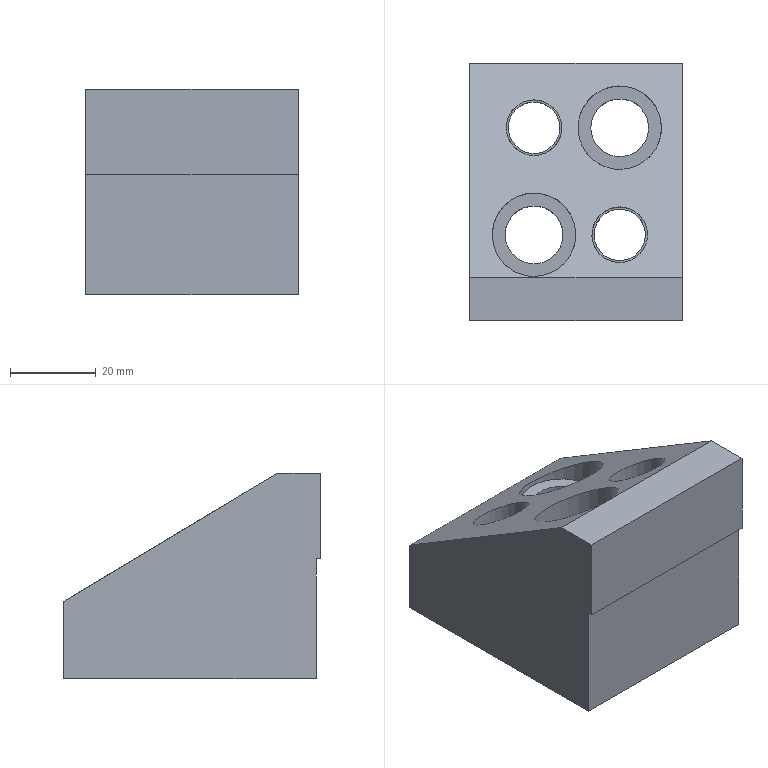Part | NX | features solid 2 | 1 solid | 21 faces | box 49.578 x 60 x 48 mm | volume 81453 mm3 | plane 13 | cylinder 8 | commonest cylinder face diameters 12 x2 13 x2 13.5 x2 19.5 x2
STEP:
#1=CARTESIAN_POINT('',(-469.,120.,-55.));
#2=VERTEX_POINT('',#1);
#3=CARTESIAN_POINT('',(-475.,120.,-55.));
#4=DIRECTION('',(0.,0.,1.));
#5=DIRECTION('',(1.,0.,0.));
#6=AXIS2_PLACEMENT_3D('',#3,#4,#5);
#7=CIRCLE('',#6,6.);
#8=EDGE_CURVE('',#2,#2,#7,.F.);
#9=ORIENTED_EDGE('',*,*,#8,.F.);
#10=EDGE_LOOP('',(#9));
#11=FACE_BOUND('',#10,.T.);
#12=CARTESIAN_POINT('',(-489.,145.,-55.));
#13=VERTEX_POINT('',#12);
#14=CARTESIAN_POINT('',(-495.,145.,-55.));
#15=DIRECTION('',(0.,0.,1.));
#16=DIRECTION('',(1.,0.,0.));
#17=AXIS2_PLACEMENT_3D('',#14,#15,#16);
#18=CIRCLE('',#17,6.);
#19=EDGE_CURVE('',#13,#13,#18,.F.);
#20=ORIENTED_EDGE('',*,*,#19,.F.);
#21=EDGE_LOOP('',(#20));
#22=FACE_BOUND('',#21,.T.);
#23=CARTESIAN_POINT('',(-468.25,145.,-55.));
#24=VERTEX_POINT('',#23);
#25=CARTESIAN_POINT('',(-475.,145.,-55.));
#26=DIRECTION('',(0.,0.,1.));
#27=DIRECTION('',(1.,0.,0.));
#28=AXIS2_PLACEMENT_3D('',#25,#26,#27);
#29=CIRCLE('',#28,6.75);
#30=EDGE_CURVE('',#24,#24,#29,.F.);
#31=ORIENTED_EDGE('',*,*,#30,.F.);
#32=EDGE_LOOP('',(#31));
#33=FACE_BOUND('',#32,.T.);
#34=CARTESIAN_POINT('',(-488.25,120.,-55.));
#35=VERTEX_POINT('',#34);
#36=CARTESIAN_POINT('',(-495.,120.,-55.));
#37=DIRECTION('',(0.,0.,1.));
#38=DIRECTION('',(1.,0.,0.));
#39=AXIS2_PLACEMENT_3D('',#36,#37,#38);
#40=CIRCLE('',#39,6.75);
#41=EDGE_CURVE('',#35,#35,#40,.F.);
#42=ORIENTED_EDGE('',*,*,#41,.F.);
#43=EDGE_LOOP('',(#42));
#44=FACE_BOUND('',#43,.T.);
#45=CARTESIAN_POINT('',(-510.,160.,-55.));
#46=VERTEX_POINT('',#45);
#47=CARTESIAN_POINT('',(-510.,101.,-55.));
#48=VERTEX_POINT('',#47);
#49=CARTESIAN_POINT('',(-510.,35.09,-55.));
#50=DIRECTION('',(0.,1.,0.));
#51=VECTOR('',#50,1000.);
#52=LINE('',#49,#51);
#53=EDGE_CURVE('',#46,#48,#52,.F.);
#54=ORIENTED_EDGE('',*,*,#53,.F.);
#55=CARTESIAN_POINT('',(-460.422,160.,-55.));
#56=VERTEX_POINT('',#55);
#57=CARTESIAN_POINT('',(-459.422,160.,-55.));
#58=DIRECTION('',(1.,0.,0.));
#59=VECTOR('',#58,1000.);
#60=LINE('',#57,#59);
#61=EDGE_CURVE('',#56,#46,#60,.F.);
#62=ORIENTED_EDGE('',*,*,#61,.F.);
#63=CARTESIAN_POINT('',(-460.422,101.,-55.));
#64=VERTEX_POINT('',#63);
#65=CARTESIAN_POINT('',(-460.422,100.,-55.));
#66=DIRECTION('',(0.,1.,0.));
#67=VECTOR('',#66,1000.);
#68=LINE('',#65,#67);
#69=EDGE_CURVE('',#64,#56,#68,.T.);
#70=ORIENTED_EDGE('',*,*,#69,.F.);
#71=CARTESIAN_POINT('',(-415.478,101.,-55.));
#72=DIRECTION('',(1.,0.,0.));
#73=VECTOR('',#72,1000.);
#74=LINE('',#71,#73);
#75=EDGE_CURVE('',#64,#48,#74,.F.);
#76=ORIENTED_EDGE('',*,*,#75,.T.);
#77=EDGE_LOOP('',(#54,#62,#70,#76));
#78=FACE_BOUND('',#77,.T.);
#79=CARTESIAN_POINT('',(-415.478,35.09,-55.));
#80=DIRECTION('',(0.,0.,1.));
#81=DIRECTION('',(1.,0.,0.));
#82=AXIS2_PLACEMENT_3D('',#79,#80,#81);
#83=PLANE('',#82);
#84=ADVANCED_FACE('',(#11,#22,#33,#44,#78),#83,.F.);
#85=CARTESIAN_POINT('',(-510.,100.,-7.));
#86=VERTEX_POINT('',#85);
#87=CARTESIAN_POINT('',(-510.,110.,-7.));
#88=VERTEX_POINT('',#87);
#89=CARTESIAN_POINT('',(-510.,100.,-7.));
#90=DIRECTION('',(0.,-1.,0.));
#91=VECTOR('',#90,1000.);
#92=LINE('',#89,#91);
#93=EDGE_CURVE('',#86,#88,#92,.F.);
#94=ORIENTED_EDGE('',*,*,#93,.F.);
#95=CARTESIAN_POINT('',(-460.422,100.,-7.));
#96=VERTEX_POINT('',#95);
#97=CARTESIAN_POINT('',(-459.422,100.,-7.));
#98=DIRECTION('',(-1.,0.,0.));
#99=VECTOR('',#98,1000.);
#100=LINE('',#97,#99);
#101=EDGE_CURVE('',#96,#86,#100,.T.);
#102=ORIENTED_EDGE('',*,*,#101,.F.);
#103=CARTESIAN_POINT('',(-460.422,110.,-7.));
#104=VERTEX_POINT('',#103);
#105=CARTESIAN_POINT('',(-460.422,100.,-7.));
#106=DIRECTION('',(0.,1.,0.));
#107=VECTOR('',#106,1000.);
#108=LINE('',#105,#107);
#109=EDGE_CURVE('',#96,#104,#108,.T.);
#110=ORIENTED_EDGE('',*,*,#109,.T.);
#111=CARTESIAN_POINT('',(-459.422,110.,-7.));
#112=DIRECTION('',(1.,0.,0.));
#113=VECTOR('',#112,1000.);
#114=LINE('',#111,#113);
#115=EDGE_CURVE('',#104,#88,#114,.F.);
#116=ORIENTED_EDGE('',*,*,#115,.T.);
#117=EDGE_LOOP('',(#94,#102,#110,#116));
#118=FACE_BOUND('',#117,.T.);
#119=CARTESIAN_POINT('',(-459.422,100.,-7.));
#120=DIRECTION('',(0.,0.,-1.));
#121=DIRECTION('',(-1.,0.,0.));
#122=AXIS2_PLACEMENT_3D('',#119,#120,#121);
#123=PLANE('',#122);
#124=ADVANCED_FACE('',(#118),#123,.F.);
#125=CARTESIAN_POINT('',(-460.422,100.,-27.));
#126=VERTEX_POINT('',#125);
#127=CARTESIAN_POINT('',(-460.422,101.,-27.));
#128=VERTEX_POINT('',#127);
#129=CARTESIAN_POINT('',(-460.422,100.,-27.));
#130=DIRECTION('',(0.,-1.,0.));
#131=VECTOR('',#130,1000.);
#132=LINE('',#129,#131);
#133=EDGE_CURVE('',#126,#128,#132,.F.);
#134=ORIENTED_EDGE('',*,*,#133,.T.);
#135=CARTESIAN_POINT('',(-460.422,101.,-67.));
#136=DIRECTION('',(0.,0.,1.));
#137=VECTOR('',#136,1000.);
#138=LINE('',#135,#137);
#139=EDGE_CURVE('',#128,#64,#138,.F.);
#140=ORIENTED_EDGE('',*,*,#139,.T.);
#141=ORIENTED_EDGE('',*,*,#69,.T.);
#142=CARTESIAN_POINT('',(-460.422,160.,-37.));
#143=VERTEX_POINT('',#142);
#144=CARTESIAN_POINT('',(-460.422,160.,-67.));
#145=DIRECTION('',(0.,0.,-1.));
#146=VECTOR('',#145,1000.);
#147=LINE('',#144,#146);
#148=EDGE_CURVE('',#56,#143,#147,.F.);
#149=ORIENTED_EDGE('',*,*,#148,.T.);
#150=CARTESIAN_POINT('',(-460.422,129.118,-18.471));
#151=DIRECTION('',(0.,0.8575,-0.5145));
#152=VECTOR('',#151,1000.);
#153=LINE('',#150,#152);
#154=EDGE_CURVE('',#143,#104,#153,.F.);
#155=ORIENTED_EDGE('',*,*,#154,.T.);
#156=ORIENTED_EDGE('',*,*,#109,.F.);
#157=CARTESIAN_POINT('',(-460.422,100.,-67.));
#158=DIRECTION('',(0.,0.,-1.));
#159=VECTOR('',#158,1000.);
#160=LINE('',#157,#159);
#161=EDGE_CURVE('',#126,#96,#160,.F.);
#162=ORIENTED_EDGE('',*,*,#161,.F.);
#163=EDGE_LOOP('',(#134,#140,#141,#149,#155,#156,#162));
#164=FACE_BOUND('',#163,.T.);
#165=CARTESIAN_POINT('',(-460.422,100.,-67.));
#166=DIRECTION('',(-1.,0.,0.));
#167=DIRECTION('',(0.,0.,1.));
#168=AXIS2_PLACEMENT_3D('',#165,#166,#167);
#169=PLANE('',#168);
#170=ADVANCED_FACE('',(#164),#169,.F.);
#171=CARTESIAN_POINT('',(-510.,160.,-37.));
#172=VERTEX_POINT('',#171);
#173=CARTESIAN_POINT('',(-510.,160.,-67.));
#174=DIRECTION('',(0.,0.,-1.));
#175=VECTOR('',#174,1000.);
#176=LINE('',#173,#175);
#177=EDGE_CURVE('',#172,#46,#176,.T.);
#178=ORIENTED_EDGE('',*,*,#177,.F.);
#179=CARTESIAN_POINT('',(-459.422,160.,-37.));
#180=DIRECTION('',(1.,0.,0.));
#181=VECTOR('',#180,1000.);
#182=LINE('',#179,#181);
#183=EDGE_CURVE('',#172,#143,#182,.T.);
#184=ORIENTED_EDGE('',*,*,#183,.T.);
#185=ORIENTED_EDGE('',*,*,#148,.F.);
#186=ORIENTED_EDGE('',*,*,#61,.T.);
#187=EDGE_LOOP('',(#178,#184,#185,#186));
#188=FACE_BOUND('',#187,.T.);
#189=CARTESIAN_POINT('',(-459.422,160.,-67.));
#190=DIRECTION('',(0.,1.,0.));
#191=DIRECTION('',(0.,0.,1.));
#192=AXIS2_PLACEMENT_3D('',#189,#190,#191);
#193=PLANE('',#192);
#194=ADVANCED_FACE('',(#188),#193,.T.);
#195=ORIENTED_EDGE('',*,*,#101,.T.);
#196=CARTESIAN_POINT('',(-510.,100.,-27.));
#197=VERTEX_POINT('',#196);
#198=CARTESIAN_POINT('',(-510.,100.,-67.));
#199=DIRECTION('',(0.,0.,-1.));
#200=VECTOR('',#199,1000.);
#201=LINE('',#198,#200);
#202=EDGE_CURVE('',#86,#197,#201,.T.);
#203=ORIENTED_EDGE('',*,*,#202,.T.);
#204=CARTESIAN_POINT('',(-459.422,100.,-27.));
#205=DIRECTION('',(1.,0.,0.));
#206=VECTOR('',#205,1000.);
#207=LINE('',#204,#206);
#208=EDGE_CURVE('',#197,#126,#207,.T.);
#209=ORIENTED_EDGE('',*,*,#208,.T.);
#210=ORIENTED_EDGE('',*,*,#161,.T.);
#211=EDGE_LOOP('',(#195,#203,#209,#210));
#212=FACE_BOUND('',#211,.T.);
#213=CARTESIAN_POINT('',(-459.422,100.,-67.));
#214=DIRECTION('',(0.,1.,0.));
#215=DIRECTION('',(0.,0.,1.));
#216=AXIS2_PLACEMENT_3D('',#213,#214,#215);
#217=PLANE('',#216);
#218=ADVANCED_FACE('',(#212),#217,.F.);
#219=CARTESIAN_POINT('',(-475.,113.5,-9.1));
#220=VERTEX_POINT('',#219);
#221=CARTESIAN_POINT('',(-475.,120.,-13.));
#222=DIRECTION('',(0.,0.5145,0.8575));
#223=DIRECTION('',(0.,-0.8575,0.5145));
#224=AXIS2_PLACEMENT_3D('',#221,#222,#223);
#225=ELLIPSE('',#224,7.58,6.5);
#226=EDGE_CURVE('',#220,#220,#225,.T.);
#227=ORIENTED_EDGE('',*,*,#226,.F.);
#228=EDGE_LOOP('',(#227));
#229=FACE_BOUND('',#228,.T.);
#230=CARTESIAN_POINT('',(-495.,138.5,-24.1));
#231=VERTEX_POINT('',#230);
#232=CARTESIAN_POINT('',(-495.,145.,-28.));
#233=DIRECTION('',(0.,0.5145,0.8575));
#234=DIRECTION('',(0.,-0.8575,0.5145));
#235=AXIS2_PLACEMENT_3D('',#232,#233,#234);
#236=ELLIPSE('',#235,7.58,6.5);
#237=EDGE_CURVE('',#231,#231,#236,.T.);
#238=ORIENTED_EDGE('',*,*,#237,.F.);
#239=EDGE_LOOP('',(#238));
#240=FACE_BOUND('',#239,.T.);
#241=CARTESIAN_POINT('',(-475.,135.25,-22.15));
#242=VERTEX_POINT('',#241);
#243=CARTESIAN_POINT('',(-475.,145.,-28.));
#244=DIRECTION('',(0.,0.5145,0.8575));
#245=DIRECTION('',(0.,-0.8575,0.5145));
#246=AXIS2_PLACEMENT_3D('',#243,#244,#245);
#247=ELLIPSE('',#246,11.37,9.75);
#248=EDGE_CURVE('',#242,#242,#247,.T.);
#249=ORIENTED_EDGE('',*,*,#248,.F.);
#250=EDGE_LOOP('',(#249));
#251=FACE_BOUND('',#250,.T.);
#252=CARTESIAN_POINT('',(-495.,110.25,-7.15));
#253=VERTEX_POINT('',#252);
#254=CARTESIAN_POINT('',(-495.,120.,-13.));
#255=DIRECTION('',(0.,0.5145,0.8575));
#256=DIRECTION('',(0.,-0.8575,0.5145));
#257=AXIS2_PLACEMENT_3D('',#254,#255,#256);
#258=ELLIPSE('',#257,11.37,9.75);
#259=EDGE_CURVE('',#253,#253,#258,.T.);
#260=ORIENTED_EDGE('',*,*,#259,.F.);
#261=EDGE_LOOP('',(#260));
#262=FACE_BOUND('',#261,.T.);
#263=CARTESIAN_POINT('',(-510.,110.,-7.));
#264=DIRECTION('',(0.,0.8575,-0.5145));
#265=VECTOR('',#264,1000.);
#266=LINE('',#263,#265);
#267=EDGE_CURVE('',#88,#172,#266,.T.);
#268=ORIENTED_EDGE('',*,*,#267,.F.);
#269=ORIENTED_EDGE('',*,*,#115,.F.);
#270=ORIENTED_EDGE('',*,*,#154,.F.);
#271=ORIENTED_EDGE('',*,*,#183,.F.);
#272=EDGE_LOOP('',(#268,#269,#270,#271));
#273=FACE_BOUND('',#272,.T.);
#274=CARTESIAN_POINT('',(-480.376,110.,-7.));
#275=DIRECTION('',(0.,0.5145,0.8575));
#276=DIRECTION('',(0.,-0.8575,0.5145));
#277=AXIS2_PLACEMENT_3D('',#274,#275,#276);
#278=PLANE('',#277);
#279=ADVANCED_FACE('',(#229,#240,#251,#262,#273),#278,.T.);
#280=ORIENTED_EDGE('',*,*,#208,.F.);
#281=CARTESIAN_POINT('',(-510.,101.,-27.));
#282=VERTEX_POINT('',#281);
#283=CARTESIAN_POINT('',(-510.,100.,-27.));
#284=DIRECTION('',(0.,1.,0.));
#285=VECTOR('',#284,1000.);
#286=LINE('',#283,#285);
#287=EDGE_CURVE('',#197,#282,#286,.T.);
#288=ORIENTED_EDGE('',*,*,#287,.T.);
#289=CARTESIAN_POINT('',(-459.422,101.,-27.));
#290=DIRECTION('',(1.,0.,0.));
#291=VECTOR('',#290,1000.);
#292=LINE('',#289,#291);
#293=EDGE_CURVE('',#128,#282,#292,.F.);
#294=ORIENTED_EDGE('',*,*,#293,.F.);
#295=ORIENTED_EDGE('',*,*,#133,.F.);
#296=EDGE_LOOP('',(#280,#288,#294,#295));
#297=FACE_BOUND('',#296,.T.);
#298=CARTESIAN_POINT('',(-459.422,100.,-27.));
#299=DIRECTION('',(0.,0.,1.));
#300=DIRECTION('',(-1.,0.,0.));
#301=AXIS2_PLACEMENT_3D('',#298,#299,#300);
#302=PLANE('',#301);
#303=ADVANCED_FACE('',(#297),#302,.F.);
#304=CARTESIAN_POINT('',(-510.,101.,-27.));
#305=DIRECTION('',(0.,0.,1.));
#306=VECTOR('',#305,1000.);
#307=LINE('',#304,#306);
#308=EDGE_CURVE('',#48,#282,#307,.T.);
#309=ORIENTED_EDGE('',*,*,#308,.F.);
#310=ORIENTED_EDGE('',*,*,#75,.F.);
#311=ORIENTED_EDGE('',*,*,#139,.F.);
#312=ORIENTED_EDGE('',*,*,#293,.T.);
#313=EDGE_LOOP('',(#309,#310,#311,#312));
#314=FACE_BOUND('',#313,.T.);
#315=CARTESIAN_POINT('',(-459.422,101.,-27.));
#316=DIRECTION('',(0.,-1.,0.));
#317=DIRECTION('',(0.,0.,-1.));
#318=AXIS2_PLACEMENT_3D('',#315,#316,#317);
#319=PLANE('',#318);
#320=ADVANCED_FACE('',(#314),#319,.T.);
#321=ORIENTED_EDGE('',*,*,#267,.T.);
#322=ORIENTED_EDGE('',*,*,#177,.T.);
#323=ORIENTED_EDGE('',*,*,#53,.T.);
#324=ORIENTED_EDGE('',*,*,#308,.T.);
#325=ORIENTED_EDGE('',*,*,#287,.F.);
#326=ORIENTED_EDGE('',*,*,#202,.F.);
#327=ORIENTED_EDGE('',*,*,#93,.T.);
#328=EDGE_LOOP('',(#321,#322,#323,#324,#325,#326,#327));
#329=FACE_BOUND('',#328,.T.);
#330=CARTESIAN_POINT('',(-510.,0.,-7.));
#331=DIRECTION('',(1.,0.,0.));
#332=DIRECTION('',(0.,0.,-1.));
#333=AXIS2_PLACEMENT_3D('',#330,#331,#332);
#334=PLANE('',#333);
#335=ADVANCED_FACE('',(#329),#334,.F.);
#336=ORIENTED_EDGE('',*,*,#41,.T.);
#337=EDGE_LOOP('',(#336));
#338=FACE_BOUND('',#337,.T.);
#339=CARTESIAN_POINT('',(-501.75,120.,-35.));
#340=VERTEX_POINT('',#339);
#341=CARTESIAN_POINT('',(-495.,120.,-35.));
#342=DIRECTION('',(0.,0.,-1.));
#343=DIRECTION('',(-1.,0.,0.));
#344=AXIS2_PLACEMENT_3D('',#341,#342,#343);
#345=CIRCLE('',#344,6.75);
#346=EDGE_CURVE('',#340,#340,#345,.F.);
#347=ORIENTED_EDGE('',*,*,#346,.T.);
#348=EDGE_LOOP('',(#347));
#349=FACE_BOUND('',#348,.T.);
#350=CARTESIAN_POINT('',(-495.,120.,-75.));
#351=DIRECTION('',(0.,0.,1.));
#352=DIRECTION('',(1.,0.,0.));
#353=AXIS2_PLACEMENT_3D('',#350,#351,#352);
#354=CYLINDRICAL_SURFACE('',#353,6.75);
#355=ADVANCED_FACE('',(#338,#349),#354,.F.);
#356=ORIENTED_EDGE('',*,*,#346,.F.);
#357=EDGE_LOOP('',(#356));
#358=FACE_BOUND('',#357,.T.);
#359=CARTESIAN_POINT('',(-485.25,120.,-35.));
#360=VERTEX_POINT('',#359);
#361=CARTESIAN_POINT('',(-495.,120.,-35.));
#362=DIRECTION('',(0.,0.,1.));
#363=DIRECTION('',(1.,0.,0.));
#364=AXIS2_PLACEMENT_3D('',#361,#362,#363);
#365=CIRCLE('',#364,9.75);
#366=EDGE_CURVE('',#360,#360,#365,.T.);
#367=ORIENTED_EDGE('',*,*,#366,.T.);
#368=EDGE_LOOP('',(#367));
#369=FACE_BOUND('',#368,.T.);
#370=CARTESIAN_POINT('',(-495.,120.,-35.));
#371=DIRECTION('',(0.,0.,-1.));
#372=DIRECTION('',(-1.,0.,0.));
#373=AXIS2_PLACEMENT_3D('',#370,#371,#372);
#374=PLANE('',#373);
#375=ADVANCED_FACE('',(#358,#369),#374,.F.);
#376=ORIENTED_EDGE('',*,*,#259,.T.);
#377=EDGE_LOOP('',(#376));
#378=FACE_BOUND('',#377,.T.);
#379=ORIENTED_EDGE('',*,*,#366,.F.);
#380=EDGE_LOOP('',(#379));
#381=FACE_BOUND('',#380,.T.);
#382=CARTESIAN_POINT('',(-495.,120.,-35.));
#383=DIRECTION('',(0.,0.,1.));
#384=DIRECTION('',(1.,0.,0.));
#385=AXIS2_PLACEMENT_3D('',#382,#383,#384);
#386=CYLINDRICAL_SURFACE('',#385,9.75);
#387=ADVANCED_FACE('',(#378,#381),#386,.F.);
#388=ORIENTED_EDGE('',*,*,#30,.T.);
#389=EDGE_LOOP('',(#388));
#390=FACE_BOUND('',#389,.T.);
#391=CARTESIAN_POINT('',(-481.75,145.,-35.));
#392=VERTEX_POINT('',#391);
#393=CARTESIAN_POINT('',(-475.,145.,-35.));
#394=DIRECTION('',(0.,0.,-1.));
#395=DIRECTION('',(-1.,0.,0.));
#396=AXIS2_PLACEMENT_3D('',#393,#394,#395);
#397=CIRCLE('',#396,6.75);
#398=EDGE_CURVE('',#392,#392,#397,.F.);
#399=ORIENTED_EDGE('',*,*,#398,.T.);
#400=EDGE_LOOP('',(#399));
#401=FACE_BOUND('',#400,.T.);
#402=CARTESIAN_POINT('',(-475.,145.,-75.));
#403=DIRECTION('',(0.,0.,1.));
#404=DIRECTION('',(1.,0.,0.));
#405=AXIS2_PLACEMENT_3D('',#402,#403,#404);
#406=CYLINDRICAL_SURFACE('',#405,6.75);
#407=ADVANCED_FACE('',(#390,#401),#406,.F.);
#408=ORIENTED_EDGE('',*,*,#398,.F.);
#409=EDGE_LOOP('',(#408));
#410=FACE_BOUND('',#409,.T.);
#411=CARTESIAN_POINT('',(-465.25,145.,-35.));
#412=VERTEX_POINT('',#411);
#413=CARTESIAN_POINT('',(-475.,145.,-35.));
#414=DIRECTION('',(0.,0.,1.));
#415=DIRECTION('',(1.,0.,0.));
#416=AXIS2_PLACEMENT_3D('',#413,#414,#415);
#417=CIRCLE('',#416,9.75);
#418=EDGE_CURVE('',#412,#412,#417,.T.);
#419=ORIENTED_EDGE('',*,*,#418,.T.);
#420=EDGE_LOOP('',(#419));
#421=FACE_BOUND('',#420,.T.);
#422=CARTESIAN_POINT('',(-475.,145.,-35.));
#423=DIRECTION('',(0.,0.,-1.));
#424=DIRECTION('',(-1.,0.,0.));
#425=AXIS2_PLACEMENT_3D('',#422,#423,#424);
#426=PLANE('',#425);
#427=ADVANCED_FACE('',(#410,#421),#426,.F.);
#428=ORIENTED_EDGE('',*,*,#248,.T.);
#429=EDGE_LOOP('',(#428));
#430=FACE_BOUND('',#429,.T.);
#431=ORIENTED_EDGE('',*,*,#418,.F.);
#432=EDGE_LOOP('',(#431));
#433=FACE_BOUND('',#432,.T.);
#434=CARTESIAN_POINT('',(-475.,145.,-35.));
#435=DIRECTION('',(0.,0.,1.));
#436=DIRECTION('',(1.,0.,0.));
#437=AXIS2_PLACEMENT_3D('',#434,#435,#436);
#438=CYLINDRICAL_SURFACE('',#437,9.75);
#439=ADVANCED_FACE('',(#430,#433),#438,.F.);
#440=ORIENTED_EDGE('',*,*,#19,.T.);
#441=EDGE_LOOP('',(#440));
#442=FACE_BOUND('',#441,.T.);
#443=CARTESIAN_POINT('',(-501.,145.,-35.));
#444=VERTEX_POINT('',#443);
#445=CARTESIAN_POINT('',(-495.,145.,-35.));
#446=DIRECTION('',(0.,0.,-1.));
#447=DIRECTION('',(-1.,0.,0.));
#448=AXIS2_PLACEMENT_3D('',#445,#446,#447);
#449=CIRCLE('',#448,6.);
#450=EDGE_CURVE('',#444,#444,#449,.F.);
#451=ORIENTED_EDGE('',*,*,#450,.T.);
#452=EDGE_LOOP('',(#451));
#453=FACE_BOUND('',#452,.T.);
#454=CARTESIAN_POINT('',(-495.,145.,-75.));
#455=DIRECTION('',(0.,0.,1.));
#456=DIRECTION('',(1.,0.,0.));
#457=AXIS2_PLACEMENT_3D('',#454,#455,#456);
#458=CYLINDRICAL_SURFACE('',#457,6.);
#459=ADVANCED_FACE('',(#442,#453),#458,.F.);
#460=ORIENTED_EDGE('',*,*,#450,.F.);
#461=EDGE_LOOP('',(#460));
#462=FACE_BOUND('',#461,.T.);
#463=CARTESIAN_POINT('',(-488.5,145.,-35.));
#464=VERTEX_POINT('',#463);
#465=CARTESIAN_POINT('',(-495.,145.,-35.));
#466=DIRECTION('',(0.,0.,1.));
#467=DIRECTION('',(1.,0.,0.));
#468=AXIS2_PLACEMENT_3D('',#465,#466,#467);
#469=CIRCLE('',#468,6.5);
#470=EDGE_CURVE('',#464,#464,#469,.T.);
#471=ORIENTED_EDGE('',*,*,#470,.T.);
#472=EDGE_LOOP('',(#471));
#473=FACE_BOUND('',#472,.T.);
#474=CARTESIAN_POINT('',(-495.,145.,-35.));
#475=DIRECTION('',(0.,0.,-1.));
#476=DIRECTION('',(-1.,0.,0.));
#477=AXIS2_PLACEMENT_3D('',#474,#475,#476);
#478=PLANE('',#477);
#479=ADVANCED_FACE('',(#462,#473),#478,.F.);
#480=ORIENTED_EDGE('',*,*,#237,.T.);
#481=EDGE_LOOP('',(#480));
#482=FACE_BOUND('',#481,.T.);
#483=ORIENTED_EDGE('',*,*,#470,.F.);
#484=EDGE_LOOP('',(#483));
#485=FACE_BOUND('',#484,.T.);
#486=CARTESIAN_POINT('',(-495.,145.,-35.));
#487=DIRECTION('',(0.,0.,1.));
#488=DIRECTION('',(1.,0.,0.));
#489=AXIS2_PLACEMENT_3D('',#486,#487,#488);
#490=CYLINDRICAL_SURFACE('',#489,6.5);
#491=ADVANCED_FACE('',(#482,#485),#490,.F.);
#492=ORIENTED_EDGE('',*,*,#8,.T.);
#493=EDGE_LOOP('',(#492));
#494=FACE_BOUND('',#493,.T.);
#495=CARTESIAN_POINT('',(-481.,120.,-35.));
#496=VERTEX_POINT('',#495);
#497=CARTESIAN_POINT('',(-475.,120.,-35.));
#498=DIRECTION('',(0.,0.,-1.));
#499=DIRECTION('',(-1.,0.,0.));
#500=AXIS2_PLACEMENT_3D('',#497,#498,#499);
#501=CIRCLE('',#500,6.);
#502=EDGE_CURVE('',#496,#496,#501,.F.);
#503=ORIENTED_EDGE('',*,*,#502,.T.);
#504=EDGE_LOOP('',(#503));
#505=FACE_BOUND('',#504,.T.);
#506=CARTESIAN_POINT('',(-475.,120.,-75.));
#507=DIRECTION('',(0.,0.,1.));
#508=DIRECTION('',(1.,0.,0.));
#509=AXIS2_PLACEMENT_3D('',#506,#507,#508);
#510=CYLINDRICAL_SURFACE('',#509,6.);
#511=ADVANCED_FACE('',(#494,#505),#510,.F.);
#512=ORIENTED_EDGE('',*,*,#502,.F.);
#513=EDGE_LOOP('',(#512));
#514=FACE_BOUND('',#513,.T.);
#515=CARTESIAN_POINT('',(-468.5,120.,-35.));
#516=VERTEX_POINT('',#515);
#517=CARTESIAN_POINT('',(-475.,120.,-35.));
#518=DIRECTION('',(0.,0.,1.));
#519=DIRECTION('',(1.,0.,0.));
#520=AXIS2_PLACEMENT_3D('',#517,#518,#519);
#521=CIRCLE('',#520,6.5);
#522=EDGE_CURVE('',#516,#516,#521,.T.);
#523=ORIENTED_EDGE('',*,*,#522,.T.);
#524=EDGE_LOOP('',(#523));
#525=FACE_BOUND('',#524,.T.);
#526=CARTESIAN_POINT('',(-475.,120.,-35.));
#527=DIRECTION('',(0.,0.,-1.));
#528=DIRECTION('',(-1.,0.,0.));
#529=AXIS2_PLACEMENT_3D('',#526,#527,#528);
#530=PLANE('',#529);
#531=ADVANCED_FACE('',(#514,#525),#530,.F.);
#532=ORIENTED_EDGE('',*,*,#226,.T.);
#533=EDGE_LOOP('',(#532));
#534=FACE_BOUND('',#533,.T.);
#535=ORIENTED_EDGE('',*,*,#522,.F.);
#536=EDGE_LOOP('',(#535));
#537=FACE_BOUND('',#536,.T.);
#538=CARTESIAN_POINT('',(-475.,120.,-35.));
#539=DIRECTION('',(0.,0.,1.));
#540=DIRECTION('',(1.,0.,0.));
#541=AXIS2_PLACEMENT_3D('',#538,#539,#540);
#542=CYLINDRICAL_SURFACE('',#541,6.5);
#543=ADVANCED_FACE('',(#534,#537),#542,.F.);
#544=CLOSED_SHELL('',(#84,#124,#170,#194,#218,#279,#303,#320,#335,#355,#375,#387,#407,#427,#439,#459,#479,#491,#511,#531,#543));
#545=MANIFOLD_SOLID_BREP('',#544);
#546=(LENGTH_UNIT()NAMED_UNIT(*)SI_UNIT(.MILLI.,.METRE.));
#547=UNCERTAINTY_MEASURE_WITH_UNIT(LENGTH_MEASURE(0.00001),#546,'','');
#548=(NAMED_UNIT(*)PLANE_ANGLE_UNIT()SI_UNIT($,.RADIAN.));
#549=(NAMED_UNIT(*)SI_UNIT($,.STERADIAN.)SOLID_ANGLE_UNIT());
#550=(GEOMETRIC_REPRESENTATION_CONTEXT(3)GLOBAL_UNCERTAINTY_ASSIGNED_CONTEXT((#547))GLOBAL_UNIT_ASSIGNED_CONTEXT((#546,#548,#549))REPRESENTATION_CONTEXT('',''));
#551=ADVANCED_BREP_SHAPE_REPRESENTATION('',(#545),#550);